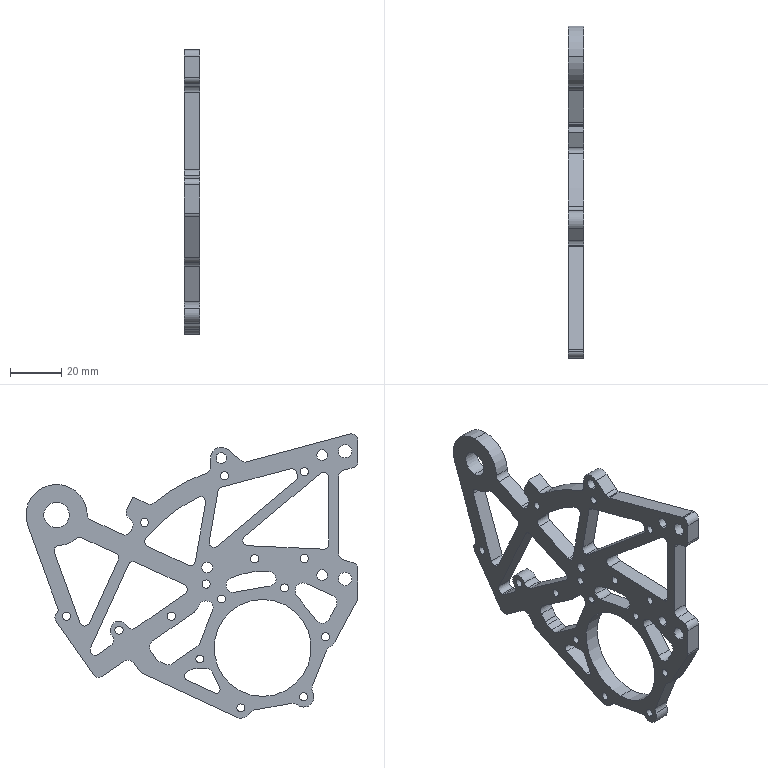Part | SolidWorks | features ICE 4, Fillet 3, Extrusion 1 | 1 solid | 184 faces | box 6 x 130 x 111.291 mm | volume 30110 mm3 | cylinder 133 | plane 51 | commonest cylinder face diameters 6 x26 4 x23 5 x21 3.2 x18 3.1 x12 4.2 x8